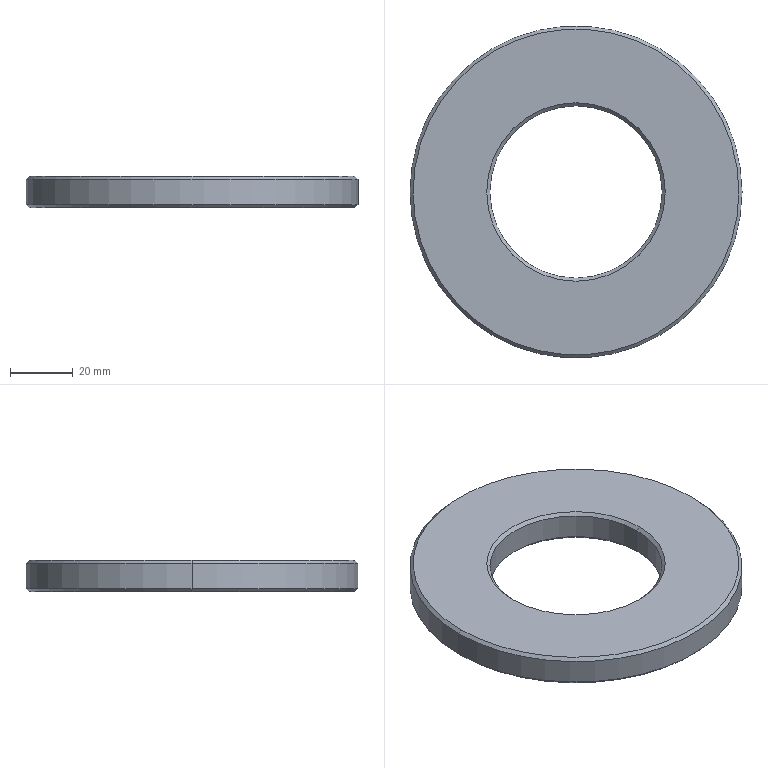Part | SolidWorks | features Chamfer 1, Extrusion 1 | 1 solid | 14 faces | box 106 x 106 x 10 mm | volume 63983 mm3 | cone 8 | cylinder 4 | plane 2 | commonest cylinder face diameters 55 x2 106 x2
STEP:
#1=CARTESIAN_POINT('',(-27.5,0.,9.));
#2=VERTEX_POINT('',#1);
#3=CARTESIAN_POINT('',(27.5,0.,9.));
#4=VERTEX_POINT('',#3);
#5=CARTESIAN_POINT('',(0.,0.,9.));
#6=DIRECTION('',(0.,0.,1.));
#7=DIRECTION('',(1.,0.,0.));
#8=AXIS2_PLACEMENT_3D('',#5,#6,#7);
#9=CIRCLE('',#8,27.5);
#10=EDGE_CURVE('',#2,#4,#9,.T.);
#11=ORIENTED_EDGE('',*,*,#10,.F.);
#12=CARTESIAN_POINT('',(-28.5,0.,10.));
#13=VERTEX_POINT('',#12);
#14=CARTESIAN_POINT('',(-27.5,0.,9.));
#15=DIRECTION('',(-0.7071,0.,0.7071));
#16=VECTOR('',#15,1000.);
#17=LINE('',#14,#16);
#18=EDGE_CURVE('',#2,#13,#17,.T.);
#19=ORIENTED_EDGE('',*,*,#18,.T.);
#20=CARTESIAN_POINT('',(28.5,0.,10.));
#21=VERTEX_POINT('',#20);
#22=CARTESIAN_POINT('',(0.,0.,10.));
#23=DIRECTION('',(0.,0.,-1.));
#24=DIRECTION('',(1.,0.,0.));
#25=AXIS2_PLACEMENT_3D('',#22,#23,#24);
#26=CIRCLE('',#25,28.5);
#27=EDGE_CURVE('',#21,#13,#26,.T.);
#28=ORIENTED_EDGE('',*,*,#27,.F.);
#29=CARTESIAN_POINT('',(27.5,0.,9.));
#30=DIRECTION('',(0.7071,0.,0.7071));
#31=VECTOR('',#30,1000.);
#32=LINE('',#29,#31);
#33=EDGE_CURVE('',#4,#21,#32,.T.);
#34=ORIENTED_EDGE('',*,*,#33,.F.);
#35=EDGE_LOOP('',(#11,#19,#28,#34));
#36=FACE_OUTER_BOUND('',#35,.T.);
#37=CARTESIAN_POINT('',(0.,0.,9.));
#38=DIRECTION('',(0.,0.,1.));
#39=DIRECTION('',(1.,0.,0.));
#40=AXIS2_PLACEMENT_3D('',#37,#38,#39);
#41=CONICAL_SURFACE('',#40,27.5,0.7854);
#42=ADVANCED_FACE('',(#36),#41,.F.);
#43=CARTESIAN_POINT('',(27.5,0.,1.));
#44=VERTEX_POINT('',#43);
#45=CARTESIAN_POINT('',(-27.5,0.,1.));
#46=VERTEX_POINT('',#45);
#47=CARTESIAN_POINT('',(0.,0.,1.));
#48=DIRECTION('',(0.,0.,-1.));
#49=DIRECTION('',(1.,0.,0.));
#50=AXIS2_PLACEMENT_3D('',#47,#48,#49);
#51=CIRCLE('',#50,27.5);
#52=EDGE_CURVE('',#44,#46,#51,.T.);
#53=ORIENTED_EDGE('',*,*,#52,.F.);
#54=CARTESIAN_POINT('',(28.5,0.,0.));
#55=VERTEX_POINT('',#54);
#56=CARTESIAN_POINT('',(28.5,0.,0.));
#57=DIRECTION('',(0.7071,0.,-0.7071));
#58=VECTOR('',#57,1000.);
#59=LINE('',#56,#58);
#60=EDGE_CURVE('',#44,#55,#59,.T.);
#61=ORIENTED_EDGE('',*,*,#60,.T.);
#62=CARTESIAN_POINT('',(-28.5,0.,0.));
#63=VERTEX_POINT('',#62);
#64=CARTESIAN_POINT('',(0.,0.,0.));
#65=DIRECTION('',(0.,0.,1.));
#66=DIRECTION('',(1.,0.,0.));
#67=AXIS2_PLACEMENT_3D('',#64,#65,#66);
#68=CIRCLE('',#67,28.5);
#69=EDGE_CURVE('',#63,#55,#68,.T.);
#70=ORIENTED_EDGE('',*,*,#69,.F.);
#71=CARTESIAN_POINT('',(-28.5,0.,0.));
#72=DIRECTION('',(-0.7071,0.,-0.7071));
#73=VECTOR('',#72,1000.);
#74=LINE('',#71,#73);
#75=EDGE_CURVE('',#46,#63,#74,.T.);
#76=ORIENTED_EDGE('',*,*,#75,.F.);
#77=EDGE_LOOP('',(#53,#61,#70,#76));
#78=FACE_OUTER_BOUND('',#77,.T.);
#79=CARTESIAN_POINT('',(0.,0.,0.));
#80=DIRECTION('',(0.,0.,-1.));
#81=DIRECTION('',(-1.,0.,0.));
#82=AXIS2_PLACEMENT_3D('',#79,#80,#81);
#83=CONICAL_SURFACE('',#82,28.5,0.7854);
#84=ADVANCED_FACE('',(#78),#83,.F.);
#85=CARTESIAN_POINT('',(52.,0.,10.));
#86=VERTEX_POINT('',#85);
#87=CARTESIAN_POINT('',(-52.,0.,10.));
#88=VERTEX_POINT('',#87);
#89=CARTESIAN_POINT('',(0.,0.,10.));
#90=DIRECTION('',(0.,0.,1.));
#91=DIRECTION('',(1.,0.,0.));
#92=AXIS2_PLACEMENT_3D('',#89,#90,#91);
#93=CIRCLE('',#92,52.);
#94=EDGE_CURVE('',#86,#88,#93,.T.);
#95=ORIENTED_EDGE('',*,*,#94,.F.);
#96=CARTESIAN_POINT('',(53.,0.,9.));
#97=VERTEX_POINT('',#96);
#98=CARTESIAN_POINT('',(52.,0.,10.));
#99=DIRECTION('',(0.7071,0.,-0.7071));
#100=VECTOR('',#99,1000.);
#101=LINE('',#98,#100);
#102=EDGE_CURVE('',#86,#97,#101,.T.);
#103=ORIENTED_EDGE('',*,*,#102,.T.);
#104=CARTESIAN_POINT('',(-53.,0.,9.));
#105=VERTEX_POINT('',#104);
#106=CARTESIAN_POINT('',(0.,0.,9.));
#107=DIRECTION('',(0.,0.,-1.));
#108=DIRECTION('',(1.,0.,0.));
#109=AXIS2_PLACEMENT_3D('',#106,#107,#108);
#110=CIRCLE('',#109,53.);
#111=EDGE_CURVE('',#105,#97,#110,.T.);
#112=ORIENTED_EDGE('',*,*,#111,.F.);
#113=CARTESIAN_POINT('',(-52.,0.,10.));
#114=DIRECTION('',(-0.7071,0.,-0.7071));
#115=VECTOR('',#114,1000.);
#116=LINE('',#113,#115);
#117=EDGE_CURVE('',#88,#105,#116,.T.);
#118=ORIENTED_EDGE('',*,*,#117,.F.);
#119=EDGE_LOOP('',(#95,#103,#112,#118));
#120=FACE_OUTER_BOUND('',#119,.T.);
#121=CARTESIAN_POINT('',(0.,0.,10.));
#122=DIRECTION('',(0.,0.,-1.));
#123=DIRECTION('',(-1.,0.,0.));
#124=AXIS2_PLACEMENT_3D('',#121,#122,#123);
#125=CONICAL_SURFACE('',#124,52.,0.7854);
#126=ADVANCED_FACE('',(#120),#125,.T.);
#127=CARTESIAN_POINT('',(-52.,0.,0.));
#128=VERTEX_POINT('',#127);
#129=CARTESIAN_POINT('',(52.,0.,0.));
#130=VERTEX_POINT('',#129);
#131=CARTESIAN_POINT('',(0.,0.,0.));
#132=DIRECTION('',(0.,0.,-1.));
#133=DIRECTION('',(1.,0.,0.));
#134=AXIS2_PLACEMENT_3D('',#131,#132,#133);
#135=CIRCLE('',#134,52.);
#136=EDGE_CURVE('',#128,#130,#135,.T.);
#137=ORIENTED_EDGE('',*,*,#136,.F.);
#138=CARTESIAN_POINT('',(-53.,0.,1.));
#139=VERTEX_POINT('',#138);
#140=CARTESIAN_POINT('',(-53.,0.,1.));
#141=DIRECTION('',(-0.7071,0.,0.7071));
#142=VECTOR('',#141,1000.);
#143=LINE('',#140,#142);
#144=EDGE_CURVE('',#128,#139,#143,.T.);
#145=ORIENTED_EDGE('',*,*,#144,.T.);
#146=CARTESIAN_POINT('',(53.,0.,1.));
#147=VERTEX_POINT('',#146);
#148=CARTESIAN_POINT('',(0.,0.,1.));
#149=DIRECTION('',(0.,0.,1.));
#150=DIRECTION('',(1.,0.,0.));
#151=AXIS2_PLACEMENT_3D('',#148,#149,#150);
#152=CIRCLE('',#151,53.);
#153=EDGE_CURVE('',#147,#139,#152,.T.);
#154=ORIENTED_EDGE('',*,*,#153,.F.);
#155=CARTESIAN_POINT('',(53.,0.,1.));
#156=DIRECTION('',(0.7071,0.,0.7071));
#157=VECTOR('',#156,1000.);
#158=LINE('',#155,#157);
#159=EDGE_CURVE('',#130,#147,#158,.T.);
#160=ORIENTED_EDGE('',*,*,#159,.F.);
#161=EDGE_LOOP('',(#137,#145,#154,#160));
#162=FACE_OUTER_BOUND('',#161,.T.);
#163=CARTESIAN_POINT('',(0.,0.,1.));
#164=DIRECTION('',(0.,0.,1.));
#165=DIRECTION('',(1.,0.,0.));
#166=AXIS2_PLACEMENT_3D('',#163,#164,#165);
#167=CONICAL_SURFACE('',#166,53.,0.7854);
#168=ADVANCED_FACE('',(#162),#167,.T.);
#169=ORIENTED_EDGE('',*,*,#10,.T.);
#170=CARTESIAN_POINT('',(27.5,0.,10.));
#171=DIRECTION('',(0.,0.,-1.));
#172=VECTOR('',#171,1000.);
#173=LINE('',#170,#172);
#174=EDGE_CURVE('',#4,#44,#173,.T.);
#175=ORIENTED_EDGE('',*,*,#174,.T.);
#176=ORIENTED_EDGE('',*,*,#52,.T.);
#177=CARTESIAN_POINT('',(-27.5,0.,10.));
#178=DIRECTION('',(0.,0.,-1.));
#179=VECTOR('',#178,1000.);
#180=LINE('',#177,#179);
#181=EDGE_CURVE('',#2,#46,#180,.T.);
#182=ORIENTED_EDGE('',*,*,#181,.F.);
#183=EDGE_LOOP('',(#169,#175,#176,#182));
#184=FACE_OUTER_BOUND('',#183,.T.);
#185=CARTESIAN_POINT('',(0.,0.,10.));
#186=DIRECTION('',(0.,0.,-1.));
#187=DIRECTION('',(-1.,0.,0.));
#188=AXIS2_PLACEMENT_3D('',#185,#186,#187);
#189=CYLINDRICAL_SURFACE('',#188,27.5);
#190=ADVANCED_FACE('',(#184),#189,.F.);
#191=ORIENTED_EDGE('',*,*,#111,.T.);
#192=CARTESIAN_POINT('',(53.,0.,10.));
#193=DIRECTION('',(0.,0.,-1.));
#194=VECTOR('',#193,1000.);
#195=LINE('',#192,#194);
#196=EDGE_CURVE('',#97,#147,#195,.T.);
#197=ORIENTED_EDGE('',*,*,#196,.T.);
#198=ORIENTED_EDGE('',*,*,#153,.T.);
#199=CARTESIAN_POINT('',(-53.,0.,10.));
#200=DIRECTION('',(0.,0.,-1.));
#201=VECTOR('',#200,1000.);
#202=LINE('',#199,#201);
#203=EDGE_CURVE('',#105,#139,#202,.T.);
#204=ORIENTED_EDGE('',*,*,#203,.F.);
#205=EDGE_LOOP('',(#191,#197,#198,#204));
#206=FACE_OUTER_BOUND('',#205,.T.);
#207=CARTESIAN_POINT('',(0.,0.,10.));
#208=DIRECTION('',(0.,0.,-1.));
#209=DIRECTION('',(-1.,0.,0.));
#210=AXIS2_PLACEMENT_3D('',#207,#208,#209);
#211=CYLINDRICAL_SURFACE('',#210,53.);
#212=ADVANCED_FACE('',(#206),#211,.T.);
#213=CARTESIAN_POINT('',(0.,0.,10.));
#214=DIRECTION('',(0.,0.,1.));
#215=DIRECTION('',(1.,0.,0.));
#216=AXIS2_PLACEMENT_3D('',#213,#214,#215);
#217=CIRCLE('',#216,52.);
#218=EDGE_CURVE('',#88,#86,#217,.T.);
#219=ORIENTED_EDGE('',*,*,#218,.T.);
#220=ORIENTED_EDGE('',*,*,#94,.T.);
#221=EDGE_LOOP('',(#219,#220));
#222=FACE_OUTER_BOUND('',#221,.T.);
#223=ORIENTED_EDGE('',*,*,#27,.T.);
#224=CARTESIAN_POINT('',(0.,0.,10.));
#225=DIRECTION('',(0.,0.,-1.));
#226=DIRECTION('',(1.,0.,0.));
#227=AXIS2_PLACEMENT_3D('',#224,#225,#226);
#228=CIRCLE('',#227,28.5);
#229=EDGE_CURVE('',#13,#21,#228,.T.);
#230=ORIENTED_EDGE('',*,*,#229,.T.);
#231=EDGE_LOOP('',(#223,#230));
#232=FACE_BOUND('',#231,.T.);
#233=CARTESIAN_POINT('',(0.,0.,10.));
#234=DIRECTION('',(0.,0.,1.));
#235=DIRECTION('',(1.,0.,0.));
#236=AXIS2_PLACEMENT_3D('',#233,#234,#235);
#237=PLANE('',#236);
#238=ADVANCED_FACE('',(#222,#232),#237,.T.);
#239=CARTESIAN_POINT('',(0.,0.,0.));
#240=DIRECTION('',(0.,0.,-1.));
#241=DIRECTION('',(1.,0.,0.));
#242=AXIS2_PLACEMENT_3D('',#239,#240,#241);
#243=CIRCLE('',#242,52.);
#244=EDGE_CURVE('',#130,#128,#243,.T.);
#245=ORIENTED_EDGE('',*,*,#244,.T.);
#246=ORIENTED_EDGE('',*,*,#136,.T.);
#247=EDGE_LOOP('',(#245,#246));
#248=FACE_OUTER_BOUND('',#247,.T.);
#249=ORIENTED_EDGE('',*,*,#69,.T.);
#250=CARTESIAN_POINT('',(0.,0.,0.));
#251=DIRECTION('',(0.,0.,1.));
#252=DIRECTION('',(1.,0.,0.));
#253=AXIS2_PLACEMENT_3D('',#250,#251,#252);
#254=CIRCLE('',#253,28.5);
#255=EDGE_CURVE('',#55,#63,#254,.T.);
#256=ORIENTED_EDGE('',*,*,#255,.T.);
#257=EDGE_LOOP('',(#249,#256));
#258=FACE_BOUND('',#257,.T.);
#259=CARTESIAN_POINT('',(0.,0.,0.));
#260=DIRECTION('',(0.,0.,1.));
#261=DIRECTION('',(1.,0.,0.));
#262=AXIS2_PLACEMENT_3D('',#259,#260,#261);
#263=PLANE('',#262);
#264=ADVANCED_FACE('',(#248,#258),#263,.F.);
#265=ORIENTED_EDGE('',*,*,#196,.F.);
#266=CARTESIAN_POINT('',(0.,0.,9.));
#267=DIRECTION('',(0.,0.,-1.));
#268=DIRECTION('',(1.,0.,0.));
#269=AXIS2_PLACEMENT_3D('',#266,#267,#268);
#270=CIRCLE('',#269,53.);
#271=EDGE_CURVE('',#97,#105,#270,.T.);
#272=ORIENTED_EDGE('',*,*,#271,.T.);
#273=ORIENTED_EDGE('',*,*,#203,.T.);
#274=CARTESIAN_POINT('',(0.,0.,1.));
#275=DIRECTION('',(0.,0.,1.));
#276=DIRECTION('',(1.,0.,0.));
#277=AXIS2_PLACEMENT_3D('',#274,#275,#276);
#278=CIRCLE('',#277,53.);
#279=EDGE_CURVE('',#139,#147,#278,.T.);
#280=ORIENTED_EDGE('',*,*,#279,.T.);
#281=EDGE_LOOP('',(#265,#272,#273,#280));
#282=FACE_OUTER_BOUND('',#281,.T.);
#283=CARTESIAN_POINT('',(0.,0.,10.));
#284=DIRECTION('',(0.,0.,-1.));
#285=DIRECTION('',(-1.,0.,0.));
#286=AXIS2_PLACEMENT_3D('',#283,#284,#285);
#287=CYLINDRICAL_SURFACE('',#286,53.);
#288=ADVANCED_FACE('',(#282),#287,.T.);
#289=ORIENTED_EDGE('',*,*,#174,.F.);
#290=CARTESIAN_POINT('',(0.,0.,9.));
#291=DIRECTION('',(0.,0.,1.));
#292=DIRECTION('',(1.,0.,0.));
#293=AXIS2_PLACEMENT_3D('',#290,#291,#292);
#294=CIRCLE('',#293,27.5);
#295=EDGE_CURVE('',#4,#2,#294,.T.);
#296=ORIENTED_EDGE('',*,*,#295,.T.);
#297=ORIENTED_EDGE('',*,*,#181,.T.);
#298=CARTESIAN_POINT('',(0.,0.,1.));
#299=DIRECTION('',(0.,0.,-1.));
#300=DIRECTION('',(1.,0.,0.));
#301=AXIS2_PLACEMENT_3D('',#298,#299,#300);
#302=CIRCLE('',#301,27.5);
#303=EDGE_CURVE('',#46,#44,#302,.T.);
#304=ORIENTED_EDGE('',*,*,#303,.T.);
#305=EDGE_LOOP('',(#289,#296,#297,#304));
#306=FACE_OUTER_BOUND('',#305,.T.);
#307=CARTESIAN_POINT('',(0.,0.,10.));
#308=DIRECTION('',(0.,0.,-1.));
#309=DIRECTION('',(-1.,0.,0.));
#310=AXIS2_PLACEMENT_3D('',#307,#308,#309);
#311=CYLINDRICAL_SURFACE('',#310,27.5);
#312=ADVANCED_FACE('',(#306),#311,.F.);
#313=ORIENTED_EDGE('',*,*,#144,.F.);
#314=ORIENTED_EDGE('',*,*,#244,.F.);
#315=ORIENTED_EDGE('',*,*,#159,.T.);
#316=ORIENTED_EDGE('',*,*,#279,.F.);
#317=EDGE_LOOP('',(#313,#314,#315,#316));
#318=FACE_OUTER_BOUND('',#317,.T.);
#319=CARTESIAN_POINT('',(0.,0.,1.));
#320=DIRECTION('',(0.,0.,1.));
#321=DIRECTION('',(1.,0.,0.));
#322=AXIS2_PLACEMENT_3D('',#319,#320,#321);
#323=CONICAL_SURFACE('',#322,53.,0.7854);
#324=ADVANCED_FACE('',(#318),#323,.T.);
#325=ORIENTED_EDGE('',*,*,#102,.F.);
#326=ORIENTED_EDGE('',*,*,#218,.F.);
#327=ORIENTED_EDGE('',*,*,#117,.T.);
#328=ORIENTED_EDGE('',*,*,#271,.F.);
#329=EDGE_LOOP('',(#325,#326,#327,#328));
#330=FACE_OUTER_BOUND('',#329,.T.);
#331=CARTESIAN_POINT('',(0.,0.,10.));
#332=DIRECTION('',(0.,0.,-1.));
#333=DIRECTION('',(-1.,0.,0.));
#334=AXIS2_PLACEMENT_3D('',#331,#332,#333);
#335=CONICAL_SURFACE('',#334,52.,0.7854);
#336=ADVANCED_FACE('',(#330),#335,.T.);
#337=ORIENTED_EDGE('',*,*,#60,.F.);
#338=ORIENTED_EDGE('',*,*,#303,.F.);
#339=ORIENTED_EDGE('',*,*,#75,.T.);
#340=ORIENTED_EDGE('',*,*,#255,.F.);
#341=EDGE_LOOP('',(#337,#338,#339,#340));
#342=FACE_OUTER_BOUND('',#341,.T.);
#343=CARTESIAN_POINT('',(0.,0.,0.));
#344=DIRECTION('',(0.,0.,-1.));
#345=DIRECTION('',(-1.,0.,0.));
#346=AXIS2_PLACEMENT_3D('',#343,#344,#345);
#347=CONICAL_SURFACE('',#346,28.5,0.7854);
#348=ADVANCED_FACE('',(#342),#347,.F.);
#349=ORIENTED_EDGE('',*,*,#18,.F.);
#350=ORIENTED_EDGE('',*,*,#295,.F.);
#351=ORIENTED_EDGE('',*,*,#33,.T.);
#352=ORIENTED_EDGE('',*,*,#229,.F.);
#353=EDGE_LOOP('',(#349,#350,#351,#352));
#354=FACE_OUTER_BOUND('',#353,.T.);
#355=CARTESIAN_POINT('',(0.,0.,9.));
#356=DIRECTION('',(0.,0.,1.));
#357=DIRECTION('',(1.,0.,0.));
#358=AXIS2_PLACEMENT_3D('',#355,#356,#357);
#359=CONICAL_SURFACE('',#358,27.5,0.7854);
#360=ADVANCED_FACE('',(#354),#359,.F.);
#361=CLOSED_SHELL('',(#42,#84,#126,#168,#190,#212,#238,#264,#288,#312,#324,#336,#348,#360));
#362=MANIFOLD_SOLID_BREP('',#361);
#363=CARTESIAN_POINT('',(0.,0.,0.));
#364=DIRECTION('',(0.,0.,1.));
#365=DIRECTION('',(1.,0.,0.));
#366=AXIS2_PLACEMENT_3D('',#363,#364,#365);
#367=(LENGTH_UNIT()NAMED_UNIT(*)SI_UNIT(.MILLI.,.METRE.));
#368=UNCERTAINTY_MEASURE_WITH_UNIT(LENGTH_MEASURE(0.00001),#367,'','');
#369=(NAMED_UNIT(*)PLANE_ANGLE_UNIT()SI_UNIT($,.RADIAN.));
#370=(NAMED_UNIT(*)SI_UNIT($,.STERADIAN.)SOLID_ANGLE_UNIT());
#371=(GEOMETRIC_REPRESENTATION_CONTEXT(3)GLOBAL_UNCERTAINTY_ASSIGNED_CONTEXT((#368))GLOBAL_UNIT_ASSIGNED_CONTEXT((#367,#369,#370))REPRESENTATION_CONTEXT('',''));
#372=ADVANCED_BREP_SHAPE_REPRESENTATION('',(#362,#366),#371);